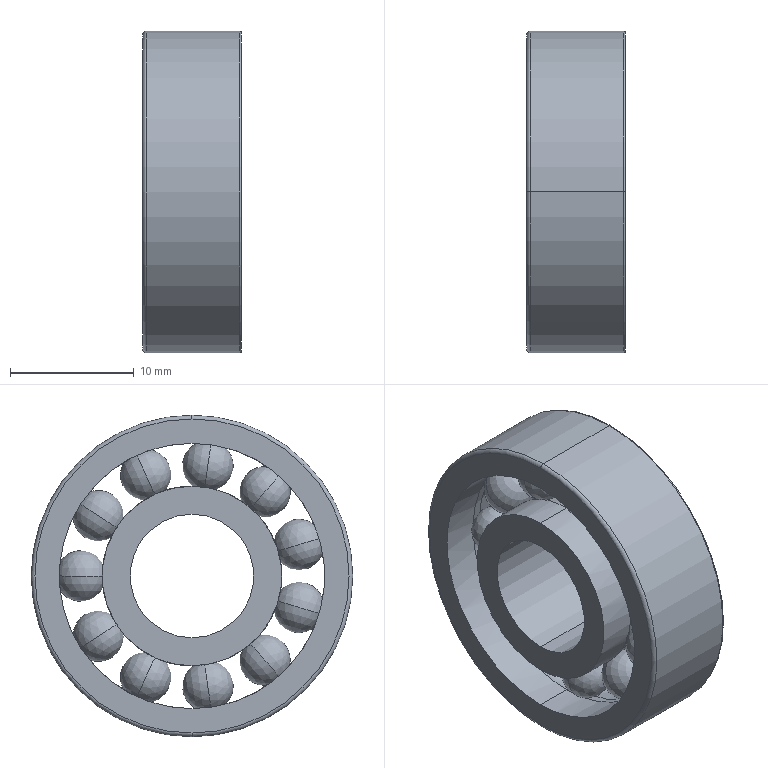Part | NX | features BREP 1 | 1 solid | 80 faces | box 8 x 26 x 26 mm | volume 2250 mm3 | torus 42 | sphere 22 | cylinder 10 | plane 4 | cone 2 | commonest cylinder face diameters 14.536 x4 10 x2 21.464 x2 26 x2